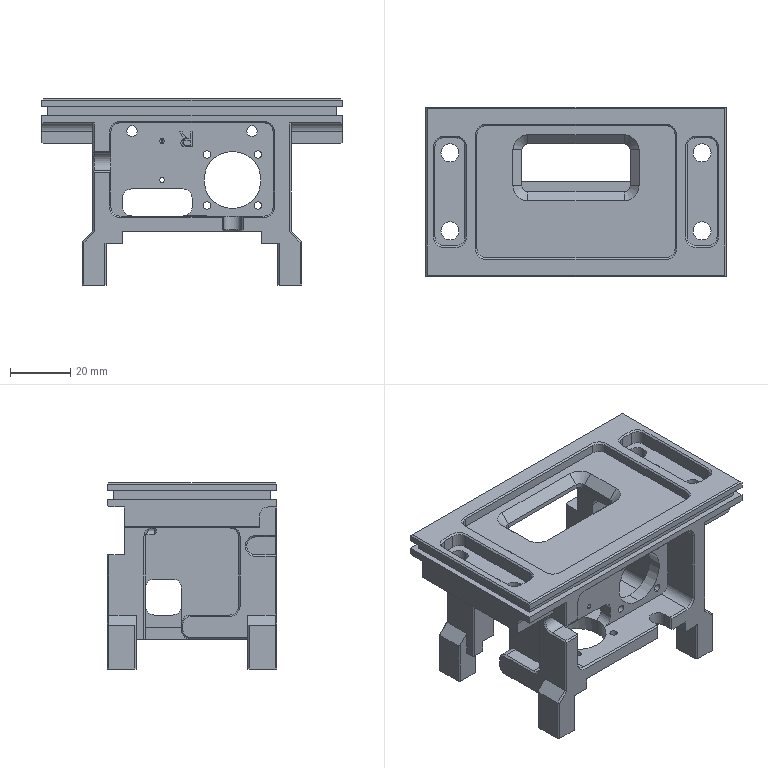NC program | Mastercam | posted with a generic post | part box 100 x 56.5 x 62 mm
Lines 1 to 33 of 45570:
%
O0000()
(MATERIAL - ALUMINUM MM - 2024)
( T20 | 63 FEM | H20 )
( T13 | 16 FEM | H13 | XY STOCK TO LEAVE - .15 | Z STOCK TO LEAVE - 0. )
( T16 | 16 FEM | H16 )
( T6 | 6 FEM | H6 | XY STOCK TO LEAVE - .1 | Z STOCK TO LEAVE - .1 )
( T2 | 2 FEM | H2 | XY STOCK TO LEAVE - .08 | Z STOCK TO LEAVE - .05 )
( T5 | 4 CHM | H5 )
( T11 | 12 FEM | H11 | XY STOCK TO LEAVE - .1 | Z STOCK TO LEAVE - .1 )
( T12 | 12 FEM | H12 )
( T14 | CO 6 FEM | H14 | XY STOCK TO LEAVE - .1 | Z STOCK TO LEAVE - .1 )
( T15 | CO 4 FEM | H15 | XY STOCK TO LEAVE - .1 | Z STOCK TO LEAVE - .05 )
( T3 | 3 FEM | H3 | XY STOCK TO LEAVE - .1 | Z STOCK TO LEAVE - 0. )
( T17 | 14 CHM | H17 )
( T4 | 4 FEM | H4 | XY STOCK TO LEAVE - .07 | Z STOCK TO LEAVE - 0. )
( T18 | CO 6 FEM | H18 | XY STOCK TO LEAVE - -.01 | Z STOCK TO LEAVE - 0. )
N100 G21
N110 G0 G17 G40 G49 G80 G90
N120 T20 M6
N130 G0 G90 G54 X-99.1 Y21.098 A0. S4000 M3
N140 G43 H20 Z20. M8
N150 Z1.
N160 G1 Z0. F600.
N170 X67.6 F1000.
N180 G2 X88.698 Y0. I0. J-21.098
N190 X67.6 Y-21.098 I-21.098 J0.
N200 G1 X-99.1
N210 G0 Z20.
N220 M5
N230 G91 G28 Z0. M9
N240 A0.
N250 M01